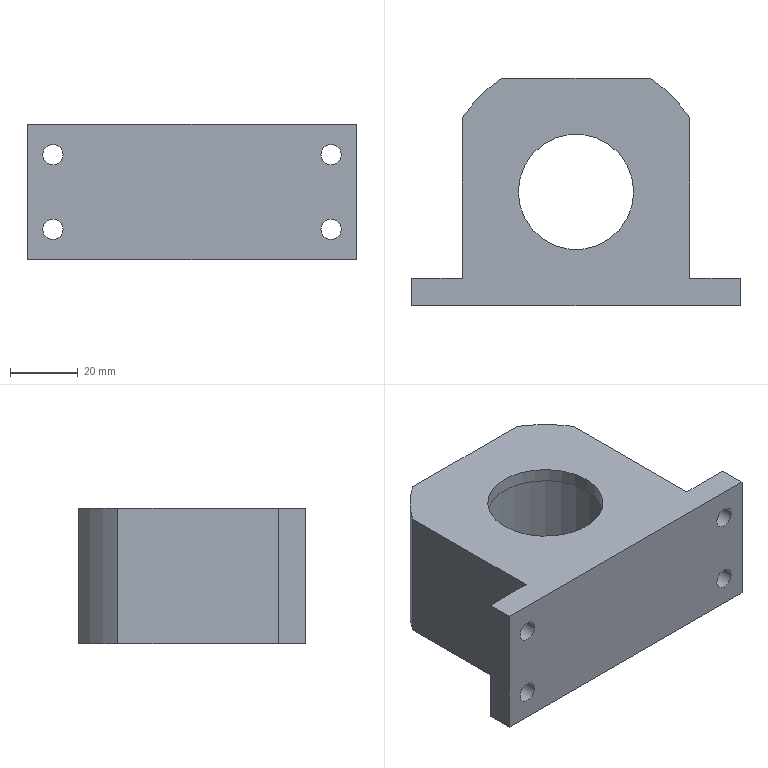Part | STEP file | Cut-off module bearing seat | 1 solid | 41 faces | box 97 x 67 x 40 mm | volume 117140 mm3 | cylinder 22 | plane 11 | cone 8 | commonest cylinder face diameters 3.3 x8 6 x8 34 x2 47 x2 80 x2
STEP:
#1=CARTESIAN_POINT('',(22.863,21.213,10.1));
#2=VERTEX_POINT('',#1);
#3=CARTESIAN_POINT('',(19.563,21.213,10.1));
#4=VERTEX_POINT('',#3);
#5=CARTESIAN_POINT('',(21.213,21.213,10.1));
#6=DIRECTION('',(0.,0.,-1.));
#7=DIRECTION('',(-1.,0.,0.));
#8=AXIS2_PLACEMENT_3D('',#5,#6,#7);
#9=CIRCLE('',#8,1.65);
#10=EDGE_CURVE('',#2,#4,#9,.T.);
#11=ORIENTED_EDGE('',*,*,#10,.F.);
#12=CARTESIAN_POINT('',(22.863,21.213,0.));
#13=VERTEX_POINT('',#12);
#14=CARTESIAN_POINT('',(22.863,21.213,0.));
#15=DIRECTION('',(0.,0.,-1.));
#16=VECTOR('',#15,1000.);
#17=LINE('',#14,#16);
#18=EDGE_CURVE('',#2,#13,#17,.T.);
#19=ORIENTED_EDGE('',*,*,#18,.T.);
#20=CARTESIAN_POINT('',(19.563,21.213,0.));
#21=VERTEX_POINT('',#20);
#22=CARTESIAN_POINT('',(21.213,21.213,0.));
#23=DIRECTION('',(0.,0.,-1.));
#24=DIRECTION('',(-1.,0.,0.));
#25=AXIS2_PLACEMENT_3D('',#22,#23,#24);
#26=CIRCLE('',#25,1.65);
#27=EDGE_CURVE('',#13,#21,#26,.T.);
#28=ORIENTED_EDGE('',*,*,#27,.T.);
#29=CARTESIAN_POINT('',(19.563,21.213,0.));
#30=DIRECTION('',(0.,0.,-1.));
#31=VECTOR('',#30,1000.);
#32=LINE('',#29,#31);
#33=EDGE_CURVE('',#4,#21,#32,.T.);
#34=ORIENTED_EDGE('',*,*,#33,.F.);
#35=EDGE_LOOP('',(#11,#19,#28,#34));
#36=FACE_OUTER_BOUND('',#35,.T.);
#37=CARTESIAN_POINT('',(21.213,21.213,0.));
#38=DIRECTION('',(0.,0.,-1.));
#39=DIRECTION('',(-1.,0.,0.));
#40=AXIS2_PLACEMENT_3D('',#37,#38,#39);
#41=CYLINDRICAL_SURFACE('',#40,1.65);
#42=ADVANCED_FACE('',(#36),#41,.F.);
#43=CARTESIAN_POINT('',(21.213,21.213,11.091));
#44=VERTEX_POINT('',#43);
#45=CARTESIAN_POINT('',(19.563,21.213,10.1));
#46=DIRECTION('',(-0.8572,0.,-0.515));
#47=VECTOR('',#46,1000.);
#48=LINE('',#45,#47);
#49=EDGE_CURVE('',#44,#4,#48,.T.);
#50=ORIENTED_EDGE('',*,*,#49,.F.);
#51=CARTESIAN_POINT('',(22.863,21.213,10.1));
#52=DIRECTION('',(0.8572,0.,-0.515));
#53=VECTOR('',#52,1000.);
#54=LINE('',#51,#53);
#55=EDGE_CURVE('',#44,#2,#54,.T.);
#56=ORIENTED_EDGE('',*,*,#55,.T.);
#57=ORIENTED_EDGE('',*,*,#10,.T.);
#58=EDGE_LOOP('',(#50,#56,#57));
#59=FACE_OUTER_BOUND('',#58,.T.);
#60=CARTESIAN_POINT('',(21.213,21.213,10.1));
#61=DIRECTION('',(0.,0.,-1.));
#62=DIRECTION('',(-1.,0.,0.));
#63=AXIS2_PLACEMENT_3D('',#60,#61,#62);
#64=CONICAL_SURFACE('',#63,1.65,1.03);
#65=ADVANCED_FACE('',(#59),#64,.F.);
#66=CARTESIAN_POINT('',(-19.563,21.213,10.1));
#67=VERTEX_POINT('',#66);
#68=CARTESIAN_POINT('',(-22.863,21.213,10.1));
#69=VERTEX_POINT('',#68);
#70=CARTESIAN_POINT('',(-21.213,21.213,10.1));
#71=DIRECTION('',(0.,0.,-1.));
#72=DIRECTION('',(-1.,0.,0.));
#73=AXIS2_PLACEMENT_3D('',#70,#71,#72);
#74=CIRCLE('',#73,1.65);
#75=EDGE_CURVE('',#67,#69,#74,.T.);
#76=ORIENTED_EDGE('',*,*,#75,.F.);
#77=CARTESIAN_POINT('',(-19.563,21.213,0.));
#78=VERTEX_POINT('',#77);
#79=CARTESIAN_POINT('',(-19.563,21.213,0.));
#80=DIRECTION('',(0.,0.,-1.));
#81=VECTOR('',#80,1000.);
#82=LINE('',#79,#81);
#83=EDGE_CURVE('',#67,#78,#82,.T.);
#84=ORIENTED_EDGE('',*,*,#83,.T.);
#85=CARTESIAN_POINT('',(-22.863,21.213,0.));
#86=VERTEX_POINT('',#85);
#87=CARTESIAN_POINT('',(-21.213,21.213,0.));
#88=DIRECTION('',(0.,0.,-1.));
#89=DIRECTION('',(-1.,0.,0.));
#90=AXIS2_PLACEMENT_3D('',#87,#88,#89);
#91=CIRCLE('',#90,1.65);
#92=EDGE_CURVE('',#78,#86,#91,.T.);
#93=ORIENTED_EDGE('',*,*,#92,.T.);
#94=CARTESIAN_POINT('',(-22.863,21.213,0.));
#95=DIRECTION('',(0.,0.,-1.));
#96=VECTOR('',#95,1000.);
#97=LINE('',#94,#96);
#98=EDGE_CURVE('',#69,#86,#97,.T.);
#99=ORIENTED_EDGE('',*,*,#98,.F.);
#100=EDGE_LOOP('',(#76,#84,#93,#99));
#101=FACE_OUTER_BOUND('',#100,.T.);
#102=CARTESIAN_POINT('',(-21.213,21.213,0.));
#103=DIRECTION('',(0.,0.,-1.));
#104=DIRECTION('',(-1.,0.,0.));
#105=AXIS2_PLACEMENT_3D('',#102,#103,#104);
#106=CYLINDRICAL_SURFACE('',#105,1.65);
#107=ADVANCED_FACE('',(#101),#106,.F.);
#108=CARTESIAN_POINT('',(-21.213,21.213,11.091));
#109=VERTEX_POINT('',#108);
#110=CARTESIAN_POINT('',(-22.863,21.213,10.1));
#111=DIRECTION('',(-0.8572,0.,-0.515));
#112=VECTOR('',#111,1000.);
#113=LINE('',#110,#112);
#114=EDGE_CURVE('',#109,#69,#113,.T.);
#115=ORIENTED_EDGE('',*,*,#114,.F.);
#116=CARTESIAN_POINT('',(-19.563,21.213,10.1));
#117=DIRECTION('',(0.8572,0.,-0.515));
#118=VECTOR('',#117,1000.);
#119=LINE('',#116,#118);
#120=EDGE_CURVE('',#109,#67,#119,.T.);
#121=ORIENTED_EDGE('',*,*,#120,.T.);
#122=ORIENTED_EDGE('',*,*,#75,.T.);
#123=EDGE_LOOP('',(#115,#121,#122));
#124=FACE_OUTER_BOUND('',#123,.T.);
#125=CARTESIAN_POINT('',(-21.213,21.213,10.1));
#126=DIRECTION('',(0.,0.,-1.));
#127=DIRECTION('',(-1.,0.,0.));
#128=AXIS2_PLACEMENT_3D('',#125,#126,#127);
#129=CONICAL_SURFACE('',#128,1.65,1.03);
#130=ADVANCED_FACE('',(#124),#129,.F.);
#131=CARTESIAN_POINT('',(-19.563,-21.213,10.1));
#132=VERTEX_POINT('',#131);
#133=CARTESIAN_POINT('',(-22.863,-21.213,10.1));
#134=VERTEX_POINT('',#133);
#135=CARTESIAN_POINT('',(-21.213,-21.213,10.1));
#136=DIRECTION('',(0.,0.,-1.));
#137=DIRECTION('',(-1.,0.,0.));
#138=AXIS2_PLACEMENT_3D('',#135,#136,#137);
#139=CIRCLE('',#138,1.65);
#140=EDGE_CURVE('',#132,#134,#139,.T.);
#141=ORIENTED_EDGE('',*,*,#140,.F.);
#142=CARTESIAN_POINT('',(-19.563,-21.213,0.));
#143=VERTEX_POINT('',#142);
#144=CARTESIAN_POINT('',(-19.563,-21.213,0.));
#145=DIRECTION('',(0.,0.,-1.));
#146=VECTOR('',#145,1000.);
#147=LINE('',#144,#146);
#148=EDGE_CURVE('',#132,#143,#147,.T.);
#149=ORIENTED_EDGE('',*,*,#148,.T.);
#150=CARTESIAN_POINT('',(-22.863,-21.213,0.));
#151=VERTEX_POINT('',#150);
#152=CARTESIAN_POINT('',(-21.213,-21.213,0.));
#153=DIRECTION('',(0.,0.,-1.));
#154=DIRECTION('',(-1.,0.,0.));
#155=AXIS2_PLACEMENT_3D('',#152,#153,#154);
#156=CIRCLE('',#155,1.65);
#157=EDGE_CURVE('',#143,#151,#156,.T.);
#158=ORIENTED_EDGE('',*,*,#157,.T.);
#159=CARTESIAN_POINT('',(-22.863,-21.213,0.));
#160=DIRECTION('',(0.,0.,-1.));
#161=VECTOR('',#160,1000.);
#162=LINE('',#159,#161);
#163=EDGE_CURVE('',#134,#151,#162,.T.);
#164=ORIENTED_EDGE('',*,*,#163,.F.);
#165=EDGE_LOOP('',(#141,#149,#158,#164));
#166=FACE_OUTER_BOUND('',#165,.T.);
#167=CARTESIAN_POINT('',(-21.213,-21.213,0.));
#168=DIRECTION('',(0.,0.,-1.));
#169=DIRECTION('',(-1.,0.,0.));
#170=AXIS2_PLACEMENT_3D('',#167,#168,#169);
#171=CYLINDRICAL_SURFACE('',#170,1.65);
#172=ADVANCED_FACE('',(#166),#171,.F.);
#173=CARTESIAN_POINT('',(-21.213,-21.213,11.091));
#174=VERTEX_POINT('',#173);
#175=CARTESIAN_POINT('',(-22.863,-21.213,10.1));
#176=DIRECTION('',(-0.8572,0.,-0.515));
#177=VECTOR('',#176,1000.);
#178=LINE('',#175,#177);
#179=EDGE_CURVE('',#174,#134,#178,.T.);
#180=ORIENTED_EDGE('',*,*,#179,.F.);
#181=CARTESIAN_POINT('',(-19.563,-21.213,10.1));
#182=DIRECTION('',(0.8572,0.,-0.515));
#183=VECTOR('',#182,1000.);
#184=LINE('',#181,#183);
#185=EDGE_CURVE('',#174,#132,#184,.T.);
#186=ORIENTED_EDGE('',*,*,#185,.T.);
#187=ORIENTED_EDGE('',*,*,#140,.T.);
#188=EDGE_LOOP('',(#180,#186,#187));
#189=FACE_OUTER_BOUND('',#188,.T.);
#190=CARTESIAN_POINT('',(-21.213,-21.213,10.1));
#191=DIRECTION('',(0.,0.,-1.));
#192=DIRECTION('',(-1.,0.,0.));
#193=AXIS2_PLACEMENT_3D('',#190,#191,#192);
#194=CONICAL_SURFACE('',#193,1.65,1.03);
#195=ADVANCED_FACE('',(#189),#194,.F.);
#196=CARTESIAN_POINT('',(22.863,-21.213,10.1));
#197=VERTEX_POINT('',#196);
#198=CARTESIAN_POINT('',(19.563,-21.213,10.1));
#199=VERTEX_POINT('',#198);
#200=CARTESIAN_POINT('',(21.213,-21.213,10.1));
#201=DIRECTION('',(0.,0.,-1.));
#202=DIRECTION('',(-1.,0.,0.));
#203=AXIS2_PLACEMENT_3D('',#200,#201,#202);
#204=CIRCLE('',#203,1.65);
#205=EDGE_CURVE('',#197,#199,#204,.T.);
#206=ORIENTED_EDGE('',*,*,#205,.F.);
#207=CARTESIAN_POINT('',(22.863,-21.213,0.));
#208=VERTEX_POINT('',#207);
#209=CARTESIAN_POINT('',(22.863,-21.213,0.));
#210=DIRECTION('',(0.,0.,-1.));
#211=VECTOR('',#210,1000.);
#212=LINE('',#209,#211);
#213=EDGE_CURVE('',#197,#208,#212,.T.);
#214=ORIENTED_EDGE('',*,*,#213,.T.);
#215=CARTESIAN_POINT('',(19.563,-21.213,0.));
#216=VERTEX_POINT('',#215);
#217=CARTESIAN_POINT('',(21.213,-21.213,0.));
#218=DIRECTION('',(0.,0.,-1.));
#219=DIRECTION('',(-1.,0.,0.));
#220=AXIS2_PLACEMENT_3D('',#217,#218,#219);
#221=CIRCLE('',#220,1.65);
#222=EDGE_CURVE('',#208,#216,#221,.T.);
#223=ORIENTED_EDGE('',*,*,#222,.T.);
#224=CARTESIAN_POINT('',(19.563,-21.213,0.));
#225=DIRECTION('',(0.,0.,-1.));
#226=VECTOR('',#225,1000.);
#227=LINE('',#224,#226);
#228=EDGE_CURVE('',#199,#216,#227,.T.);
#229=ORIENTED_EDGE('',*,*,#228,.F.);
#230=EDGE_LOOP('',(#206,#214,#223,#229));
#231=FACE_OUTER_BOUND('',#230,.T.);
#232=CARTESIAN_POINT('',(21.213,-21.213,0.));
#233=DIRECTION('',(0.,0.,-1.));
#234=DIRECTION('',(-1.,0.,0.));
#235=AXIS2_PLACEMENT_3D('',#232,#233,#234);
#236=CYLINDRICAL_SURFACE('',#235,1.65);
#237=ADVANCED_FACE('',(#231),#236,.F.);
#238=CARTESIAN_POINT('',(21.213,-21.213,11.091));
#239=VERTEX_POINT('',#238);
#240=CARTESIAN_POINT('',(19.563,-21.213,10.1));
#241=DIRECTION('',(-0.8572,0.,-0.515));
#242=VECTOR('',#241,1000.);
#243=LINE('',#240,#242);
#244=EDGE_CURVE('',#239,#199,#243,.T.);
#245=ORIENTED_EDGE('',*,*,#244,.F.);
#246=CARTESIAN_POINT('',(22.863,-21.213,10.1));
#247=DIRECTION('',(0.8572,0.,-0.515));
#248=VECTOR('',#247,1000.);
#249=LINE('',#246,#248);
#250=EDGE_CURVE('',#239,#197,#249,.T.);
#251=ORIENTED_EDGE('',*,*,#250,.T.);
#252=ORIENTED_EDGE('',*,*,#205,.T.);
#253=EDGE_LOOP('',(#245,#251,#252));
#254=FACE_OUTER_BOUND('',#253,.T.);
#255=CARTESIAN_POINT('',(21.213,-21.213,10.1));
#256=DIRECTION('',(0.,0.,-1.));
#257=DIRECTION('',(-1.,0.,0.));
#258=AXIS2_PLACEMENT_3D('',#255,#256,#257);
#259=CONICAL_SURFACE('',#258,1.65,1.03);
#260=ADVANCED_FACE('',(#254),#259,.F.);
#261=CARTESIAN_POINT('',(-44.,-33.5,9.));
#262=VERTEX_POINT('',#261);
#263=CARTESIAN_POINT('',(-38.,-33.5,9.));
#264=VERTEX_POINT('',#263);
#265=CARTESIAN_POINT('',(-41.,-33.5,9.));
#266=DIRECTION('',(0.,-1.,0.));
#267=DIRECTION('',(0.,0.,1.));
#268=AXIS2_PLACEMENT_3D('',#265,#266,#267);
#269=CIRCLE('',#268,3.);
#270=EDGE_CURVE('',#262,#264,#269,.T.);
#271=ORIENTED_EDGE('',*,*,#270,.T.);
#272=CARTESIAN_POINT('',(-38.,-25.5,9.));
#273=VERTEX_POINT('',#272);
#274=CARTESIAN_POINT('',(-38.,-45.5,9.));
#275=DIRECTION('',(0.,1.,0.));
#276=VECTOR('',#275,1000.);
#277=LINE('',#274,#276);
#278=EDGE_CURVE('',#264,#273,#277,.T.);
#279=ORIENTED_EDGE('',*,*,#278,.T.);
#280=CARTESIAN_POINT('',(-44.,-25.5,9.));
#281=VERTEX_POINT('',#280);
#282=CARTESIAN_POINT('',(-41.,-25.5,9.));
#283=DIRECTION('',(0.,-1.,0.));
#284=DIRECTION('',(1.,0.,0.));
#285=AXIS2_PLACEMENT_3D('',#282,#283,#284);
#286=CIRCLE('',#285,3.);
#287=EDGE_CURVE('',#281,#273,#286,.T.);
#288=ORIENTED_EDGE('',*,*,#287,.F.);
#289=CARTESIAN_POINT('',(-44.,-45.5,9.));
#290=DIRECTION('',(0.,1.,0.));
#291=VECTOR('',#290,1000.);
#292=LINE('',#289,#291);
#293=EDGE_CURVE('',#262,#281,#292,.T.);
#294=ORIENTED_EDGE('',*,*,#293,.F.);
#295=EDGE_LOOP('',(#271,#279,#288,#294));
#296=FACE_OUTER_BOUND('',#295,.T.);
#297=CARTESIAN_POINT('',(-41.,-45.5,9.));
#298=DIRECTION('',(0.,1.,0.));
#299=DIRECTION('',(-1.,0.,0.));
#300=AXIS2_PLACEMENT_3D('',#297,#298,#299);
#301=CYLINDRICAL_SURFACE('',#300,3.);
#302=ADVANCED_FACE('',(#296),#301,.F.);
#303=CARTESIAN_POINT('',(-44.,-33.5,31.));
#304=VERTEX_POINT('',#303);
#305=CARTESIAN_POINT('',(-38.,-33.5,31.));
#306=VERTEX_POINT('',#305);
#307=CARTESIAN_POINT('',(-41.,-33.5,31.));
#308=DIRECTION('',(0.,-1.,0.));
#309=DIRECTION('',(0.,0.,1.));
#310=AXIS2_PLACEMENT_3D('',#307,#308,#309);
#311=CIRCLE('',#310,3.);
#312=EDGE_CURVE('',#304,#306,#311,.T.);
#313=ORIENTED_EDGE('',*,*,#312,.T.);
#314=CARTESIAN_POINT('',(-38.,-25.5,31.));
#315=VERTEX_POINT('',#314);
#316=CARTESIAN_POINT('',(-38.,-45.5,31.));
#317=DIRECTION('',(0.,1.,0.));
#318=VECTOR('',#317,1000.);
#319=LINE('',#316,#318);
#320=EDGE_CURVE('',#306,#315,#319,.T.);
#321=ORIENTED_EDGE('',*,*,#320,.T.);
#322=CARTESIAN_POINT('',(-44.,-25.5,31.));
#323=VERTEX_POINT('',#322);
#324=CARTESIAN_POINT('',(-41.,-25.5,31.));
#325=DIRECTION('',(0.,-1.,0.));
#326=DIRECTION('',(1.,0.,0.));
#327=AXIS2_PLACEMENT_3D('',#324,#325,#326);
#328=CIRCLE('',#327,3.);
#329=EDGE_CURVE('',#323,#315,#328,.T.);
#330=ORIENTED_EDGE('',*,*,#329,.F.);
#331=CARTESIAN_POINT('',(-44.,-45.5,31.));
#332=DIRECTION('',(0.,1.,0.));
#333=VECTOR('',#332,1000.);
#334=LINE('',#331,#333);
#335=EDGE_CURVE('',#304,#323,#334,.T.);
#336=ORIENTED_EDGE('',*,*,#335,.F.);
#337=EDGE_LOOP('',(#313,#321,#330,#336));
#338=FACE_OUTER_BOUND('',#337,.T.);
#339=CARTESIAN_POINT('',(-41.,-45.5,31.));
#340=DIRECTION('',(0.,1.,0.));
#341=DIRECTION('',(-1.,0.,0.));
#342=AXIS2_PLACEMENT_3D('',#339,#340,#341);
#343=CYLINDRICAL_SURFACE('',#342,3.);
#344=ADVANCED_FACE('',(#338),#343,.F.);
#345=CARTESIAN_POINT('',(44.,-33.5,9.));
#346=VERTEX_POINT('',#345);
#347=CARTESIAN_POINT('',(38.,-33.5,9.));
#348=VERTEX_POINT('',#347);
#349=CARTESIAN_POINT('',(41.,-33.5,9.));
#350=DIRECTION('',(0.,1.,0.));
#351=DIRECTION('',(0.,0.,1.));
#352=AXIS2_PLACEMENT_3D('',#349,#350,#351);
#353=CIRCLE('',#352,3.);
#354=EDGE_CURVE('',#346,#348,#353,.T.);
#355=ORIENTED_EDGE('',*,*,#354,.F.);
#356=CARTESIAN_POINT('',(44.,-25.5,9.));
#357=VERTEX_POINT('',#356);
#358=CARTESIAN_POINT('',(44.,-45.5,9.));
#359=DIRECTION('',(0.,1.,0.));
#360=VECTOR('',#359,1000.);
#361=LINE('',#358,#360);
#362=EDGE_CURVE('',#346,#357,#361,.T.);
#363=ORIENTED_EDGE('',*,*,#362,.T.);
#364=CARTESIAN_POINT('',(38.,-25.5,9.));
#365=VERTEX_POINT('',#364);
#366=CARTESIAN_POINT('',(41.,-25.5,9.));
#367=DIRECTION('',(0.,1.,0.));
#368=DIRECTION('',(-1.,0.,0.));
#369=AXIS2_PLACEMENT_3D('',#366,#367,#368);
#370=CIRCLE('',#369,3.);
#371=EDGE_CURVE('',#357,#365,#370,.T.);
#372=ORIENTED_EDGE('',*,*,#371,.T.);
#373=CARTESIAN_POINT('',(38.,-45.5,9.));
#374=DIRECTION('',(0.,1.,0.));
#375=VECTOR('',#374,1000.);
#376=LINE('',#373,#375);
#377=EDGE_CURVE('',#348,#365,#376,.T.);
#378=ORIENTED_EDGE('',*,*,#377,.F.);
#379=EDGE_LOOP('',(#355,#363,#372,#378));
#380=FACE_OUTER_BOUND('',#379,.T.);
#381=CARTESIAN_POINT('',(41.,-45.5,9.));
#382=DIRECTION('',(0.,1.,0.));
#383=DIRECTION('',(-1.,0.,0.));
#384=AXIS2_PLACEMENT_3D('',#381,#382,#383);
#385=CYLINDRICAL_SURFACE('',#384,3.);
#386=ADVANCED_FACE('',(#380),#385,.F.);
#387=CARTESIAN_POINT('',(44.,-33.5,31.));
#388=VERTEX_POINT('',#387);
#389=CARTESIAN_POINT('',(38.,-33.5,31.));
#390=VERTEX_POINT('',#389);
#391=CARTESIAN_POINT('',(41.,-33.5,31.));
#392=DIRECTION('',(0.,1.,0.));
#393=DIRECTION('',(0.,0.,1.));
#394=AXIS2_PLACEMENT_3D('',#391,#392,#393);
#395=CIRCLE('',#394,3.);
#396=EDGE_CURVE('',#388,#390,#395,.T.);
#397=ORIENTED_EDGE('',*,*,#396,.F.);
#398=CARTESIAN_POINT('',(44.,-25.5,31.));
#399=VERTEX_POINT('',#398);
#400=CARTESIAN_POINT('',(44.,-45.5,31.));
#401=DIRECTION('',(0.,1.,0.));
#402=VECTOR('',#401,1000.);
#403=LINE('',#400,#402);
#404=EDGE_CURVE('',#388,#399,#403,.T.);
#405=ORIENTED_EDGE('',*,*,#404,.T.);
#406=CARTESIAN_POINT('',(38.,-25.5,31.));
#407=VERTEX_POINT('',#406);
#408=CARTESIAN_POINT('',(41.,-25.5,31.));
#409=DIRECTION('',(0.,1.,0.));
#410=DIRECTION('',(-1.,0.,0.));
#411=AXIS2_PLACEMENT_3D('',#408,#409,#410);
#412=CIRCLE('',#411,3.);
#413=EDGE_CURVE('',#399,#407,#412,.T.);
#414=ORIENTED_EDGE('',*,*,#413,.T.);
#415=CARTESIAN_POINT('',(38.,-45.5,31.));
#416=DIRECTION('',(0.,1.,0.));
#417=VECTOR('',#416,1000.);
#418=LINE('',#415,#417);
#419=EDGE_CURVE('',#390,#407,#418,.T.);
#420=ORIENTED_EDGE('',*,*,#419,.F.);
#421=EDGE_LOOP('',(#397,#405,#414,#420));
#422=FACE_OUTER_BOUND('',#421,.T.);
#423=CARTESIAN_POINT('',(41.,-45.5,31.));
#424=DIRECTION('',(0.,1.,0.));
#425=DIRECTION('',(-1.,0.,0.));
#426=AXIS2_PLACEMENT_3D('',#423,#424,#425);
#427=CYLINDRICAL_SURFACE('',#426,3.);
#428=ADVANCED_FACE('',(#422),#427,.F.);
#429=CARTESIAN_POINT('',(-17.,0.,36.));
#430=VERTEX_POINT('',#429);
#431=CARTESIAN_POINT('',(17.,0.,36.));
#432=VERTEX_POINT('',#431);
#433=CARTESIAN_POINT('',(0.,0.,36.));
#434=DIRECTION('',(0.,0.,1.));
#435=DIRECTION('',(1.,0.,0.));
#436=AXIS2_PLACEMENT_3D('',#433,#434,#435);
#437=CIRCLE('',#436,17.);
#438=EDGE_CURVE('',#430,#432,#437,.T.);
#439=ORIENTED_EDGE('',*,*,#438,.F.);
#440=CARTESIAN_POINT('',(-17.,0.,40.));
#441=VERTEX_POINT('',#440);
#442=CARTESIAN_POINT('',(-17.,0.,36.));
#443=DIRECTION('',(0.,0.,1.));
#444=VECTOR('',#443,1000.);
#445=LINE('',#442,#444);
#446=EDGE_CURVE('',#430,#441,#445,.T.);
#447=ORIENTED_EDGE('',*,*,#446,.T.);
#448=CARTESIAN_POINT('',(17.,0.,40.));
#449=VERTEX_POINT('',#448);
#450=CARTESIAN_POINT('',(0.,0.,40.));
#451=DIRECTION('',(0.,0.,1.));
#452=DIRECTION('',(1.,0.,0.));
#453=AXIS2_PLACEMENT_3D('',#450,#451,#452);
#454=CIRCLE('',#453,17.);
#455=EDGE_CURVE('',#441,#449,#454,.T.);
#456=ORIENTED_EDGE('',*,*,#455,.T.);
#457=CARTESIAN_POINT('',(17.,0.,36.));
#458=DIRECTION('',(0.,0.,1.));
#459=VECTOR('',#458,1000.);
#460=LINE('',#457,#459);
#461=EDGE_CURVE('',#432,#449,#460,.T.);
#462=ORIENTED_EDGE('',*,*,#461,.F.);
#463=EDGE_LOOP('',(#439,#447,#456,#462));
#464=FACE_OUTER_BOUND('',#463,.T.);
#465=CARTESIAN_POINT('',(0.,0.,36.));
#466=DIRECTION('',(0.,0.,1.));
#467=DIRECTION('',(1.,0.,0.));
#468=AXIS2_PLACEMENT_3D('',#465,#466,#467);
#469=CYLINDRICAL_SURFACE('',#468,17.);
#470=ADVANCED_FACE('',(#464),#469,.F.);
#471=CARTESIAN_POINT('',(-23.5,0.,36.));
#472=VERTEX_POINT('',#471);
#473=CARTESIAN_POINT('',(23.5,0.,36.));
#474=VERTEX_POINT('',#473);
#475=CARTESIAN_POINT('',(0.,0.,36.));
#476=DIRECTION('',(0.,0.,1.));
#477=DIRECTION('',(1.,0.,0.));
#478=AXIS2_PLACEMENT_3D('',#475,#476,#477);
#479=CIRCLE('',#478,23.5);
#480=EDGE_CURVE('',#472,#474,#479,.T.);
#481=ORIENTED_EDGE('',*,*,#480,.T.);
#482=CARTESIAN_POINT('',(23.5,0.,0.));
#483=VERTEX_POINT('',#482);
#484=CARTESIAN_POINT('',(23.5,0.,40.));
#485=DIRECTION('',(0.,0.,-1.));
#486=VECTOR('',#485,1000.);
#487=LINE('',#484,#486);
#488=EDGE_CURVE('',#474,#483,#487,.T.);
#489=ORIENTED_EDGE('',*,*,#488,.T.);
#490=CARTESIAN_POINT('',(-23.5,0.,0.));
#491=VERTEX_POINT('',#490);
#492=CARTESIAN_POINT('',(0.,0.,0.));
#493=DIRECTION('',(0.,0.,1.));
#494=DIRECTION('',(1.,0.,0.));
#495=AXIS2_PLACEMENT_3D('',#492,#493,#494);
#496=CIRCLE('',#495,23.5);
#497=EDGE_CURVE('',#491,#483,#496,.T.);
#498=ORIENTED_EDGE('',*,*,#497,.F.);
#499=CARTESIAN_POINT('',(-23.5,0.,40.));
#500=DIRECTION('',(0.,0.,-1.));
#501=VECTOR('',#500,1000.);
#502=LINE('',#499,#501);
#503=EDGE_CURVE('',#472,#491,#502,.T.);
#504=ORIENTED_EDGE('',*,*,#503,.F.);
#505=EDGE_LOOP('',(#481,#489,#498,#504));
#506=FACE_OUTER_BOUND('',#505,.T.);
#507=CARTESIAN_POINT('',(0.,0.,40.));
#508=DIRECTION('',(0.,0.,-1.));
#509=DIRECTION('',(-1.,0.,0.));
#510=AXIS2_PLACEMENT_3D('',#507,#508,#509);
#511=CYLINDRICAL_SURFACE('',#510,23.5);
#512=ADVANCED_FACE('',(#506),#511,.F.);
#513=CARTESIAN_POINT('',(0.,0.,40.));
#514=DIRECTION('',(0.,0.,1.));
#515=DIRECTION('',(1.,0.,0.));
#516=AXIS2_PLACEMENT_3D('',#513,#514,#515);
#517=CIRCLE('',#516,17.);
#518=EDGE_CURVE('',#449,#441,#517,.T.);
#519=ORIENTED_EDGE('',*,*,#518,.F.);
#520=ORIENTED_EDGE('',*,*,#455,.F.);
#521=EDGE_LOOP('',(#519,#520));
#522=FACE_BOUND('',#521,.T.);
#523=CARTESIAN_POINT('',(21.857,33.5,40.));
#524=VERTEX_POINT('',#523);
#525=CARTESIAN_POINT('',(33.5,21.857,40.));
#526=VERTEX_POINT('',#525);
#527=CARTESIAN_POINT('',(0.,0.,40.));
#528=DIRECTION('',(0.,0.,-1.));
#529=DIRECTION('',(1.,0.,0.));
#530=AXIS2_PLACEMENT_3D('',#527,#528,#529);
#531=CIRCLE('',#530,40.);
#532=EDGE_CURVE('',#524,#526,#531,.T.);
#533=ORIENTED_EDGE('',*,*,#532,.F.);
#534=CARTESIAN_POINT('',(-21.857,33.5,40.));
#535=VERTEX_POINT('',#534);
#536=CARTESIAN_POINT('',(-33.5,33.5,40.));
#537=DIRECTION('',(-1.,0.,0.));
#538=VECTOR('',#537,1000.);
#539=LINE('',#536,#538);
#540=EDGE_CURVE('',#524,#535,#539,.T.);
#541=ORIENTED_EDGE('',*,*,#540,.T.);
#542=CARTESIAN_POINT('',(-33.5,21.857,40.));
#543=VERTEX_POINT('',#542);
#544=CARTESIAN_POINT('',(0.,0.,40.));
#545=DIRECTION('',(0.,0.,-1.));
#546=DIRECTION('',(1.,0.,0.));
#547=AXIS2_PLACEMENT_3D('',#544,#545,#546);
#548=CIRCLE('',#547,40.);
#549=EDGE_CURVE('',#543,#535,#548,.T.);
#550=ORIENTED_EDGE('',*,*,#549,.F.);
#551=CARTESIAN_POINT('',(-33.5,-25.5,40.));
#552=VERTEX_POINT('',#551);
#553=CARTESIAN_POINT('',(-33.5,33.5,40.));
#554=DIRECTION('',(0.,-1.,0.));
#555=VECTOR('',#554,1000.);
#556=LINE('',#553,#555);
#557=EDGE_CURVE('',#543,#552,#556,.T.);
#558=ORIENTED_EDGE('',*,*,#557,.T.);
#559=CARTESIAN_POINT('',(-48.5,-25.5,40.));
#560=VERTEX_POINT('',#559);
#561=CARTESIAN_POINT('',(-48.5,-25.5,40.));
#562=DIRECTION('',(1.,0.,0.));
#563=VECTOR('',#562,1000.);
#564=LINE('',#561,#563);
#565=EDGE_CURVE('',#560,#552,#564,.T.);
#566=ORIENTED_EDGE('',*,*,#565,.F.);
#567=CARTESIAN_POINT('',(-48.5,-33.5,40.));
#568=VERTEX_POINT('',#567);
#569=CARTESIAN_POINT('',(-48.5,-33.5,40.));
#570=DIRECTION('',(0.,-1.,0.));
#571=VECTOR('',#570,1000.);
#572=LINE('',#569,#571);
#573=EDGE_CURVE('',#560,#568,#572,.T.);
#574=ORIENTED_EDGE('',*,*,#573,.T.);
#575=CARTESIAN_POINT('',(48.5,-33.5,40.));
#576=VERTEX_POINT('',#575);
#577=CARTESIAN_POINT('',(-33.5,-33.5,40.));
#578=DIRECTION('',(1.,0.,0.));
#579=VECTOR('',#578,1000.);
#580=LINE('',#577,#579);
#581=EDGE_CURVE('',#568,#576,#580,.T.);
#582=ORIENTED_EDGE('',*,*,#581,.T.);
#583=CARTESIAN_POINT('',(48.5,-25.5,40.));
#584=VERTEX_POINT('',#583);
#585=CARTESIAN_POINT('',(48.5,-33.5,40.));
#586=DIRECTION('',(0.,-1.,0.));
#587=VECTOR('',#586,1000.);
#588=LINE('',#585,#587);
#589=EDGE_CURVE('',#584,#576,#588,.T.);
#590=ORIENTED_EDGE('',*,*,#589,.F.);
#591=CARTESIAN_POINT('',(33.5,-25.5,40.));
#592=VERTEX_POINT('',#591);
#593=CARTESIAN_POINT('',(48.5,-25.5,40.));
#594=DIRECTION('',(-1.,0.,0.));
#595=VECTOR('',#594,1000.);
#596=LINE('',#593,#595);
#597=EDGE_CURVE('',#584,#592,#596,.T.);
#598=ORIENTED_EDGE('',*,*,#597,.T.);
#599=CARTESIAN_POINT('',(33.5,33.5,40.));
#600=DIRECTION('',(0.,1.,0.));
#601=VECTOR('',#600,1000.);
#602=LINE('',#599,#601);
#603=EDGE_CURVE('',#592,#526,#602,.T.);
#604=ORIENTED_EDGE('',*,*,#603,.T.);
#605=EDGE_LOOP('',(#533,#541,#550,#558,#566,#574,#582,#590,#598,#604));
#606=FACE_OUTER_BOUND('',#605,.T.);
#607=CARTESIAN_POINT('',(0.,0.,40.));
#608=DIRECTION('',(0.,0.,1.));
#609=DIRECTION('',(1.,0.,0.));
#610=AXIS2_PLACEMENT_3D('',#607,#608,#609);
#611=PLANE('',#610);
#612=ADVANCED_FACE('',(#522,#606),#611,.T.);
#613=CARTESIAN_POINT('',(21.213,21.213,0.));
#614=DIRECTION('',(0.,0.,-1.));
#615=DIRECTION('',(-1.,0.,0.));
#616=AXIS2_PLACEMENT_3D('',#613,#614,#615);
#617=CIRCLE('',#616,1.65);
#618=EDGE_CURVE('',#21,#13,#617,.T.);
#619=ORIENTED_EDGE('',*,*,#618,.F.);
#620=ORIENTED_EDGE('',*,*,#27,.F.);
#621=EDGE_LOOP('',(#619,#620));
#622=FACE_BOUND('',#621,.T.);
#623=CARTESIAN_POINT('',(-21.213,21.213,0.));
#624=DIRECTION('',(0.,0.,-1.));
#625=DIRECTION('',(-1.,0.,0.));
#626=AXIS2_PLACEMENT_3D('',#623,#624,#625);
#627=CIRCLE('',#626,1.65);
#628=EDGE_CURVE('',#86,#78,#627,.T.);
#629=ORIENTED_EDGE('',*,*,#628,.F.);
#630=ORIENTED_EDGE('',*,*,#92,.F.);
#631=EDGE_LOOP('',(#629,#630));
#632=FACE_BOUND('',#631,.T.);
#633=CARTESIAN_POINT('',(-21.213,-21.213,0.));
#634=DIRECTION('',(0.,0.,-1.));
#635=DIRECTION('',(-1.,0.,0.));
#636=AXIS2_PLACEMENT_3D('',#633,#634,#635);
#637=CIRCLE('',#636,1.65);
#638=EDGE_CURVE('',#151,#143,#637,.T.);
#639=ORIENTED_EDGE('',*,*,#638,.F.);
#640=ORIENTED_EDGE('',*,*,#157,.F.);
#641=EDGE_LOOP('',(#639,#640));
#642=FACE_BOUND('',#641,.T.);
#643=CARTESIAN_POINT('',(21.213,-21.213,0.));
#644=DIRECTION('',(0.,0.,-1.));
#645=DIRECTION('',(-1.,0.,0.));
#646=AXIS2_PLACEMENT_3D('',#643,#644,#645);
#647=CIRCLE('',#646,1.65);
#648=EDGE_CURVE('',#216,#208,#647,.T.);
#649=ORIENTED_EDGE('',*,*,#648,.F.);
#650=ORIENTED_EDGE('',*,*,#222,.F.);
#651=EDGE_LOOP('',(#649,#650));
#652=FACE_BOUND('',#651,.T.);
#653=ORIENTED_EDGE('',*,*,#497,.T.);
#654=CARTESIAN_POINT('',(0.,0.,0.));
#655=DIRECTION('',(0.,0.,1.));
#656=DIRECTION('',(1.,0.,0.));
#657=AXIS2_PLACEMENT_3D('',#654,#655,#656);
#658=CIRCLE('',#657,23.5);
#659=EDGE_CURVE('',#483,#491,#658,.T.);
#660=ORIENTED_EDGE('',*,*,#659,.T.);
#661=EDGE_LOOP('',(#653,#660));
#662=FACE_BOUND('',#661,.T.);
#663=CARTESIAN_POINT('',(21.857,33.5,0.));
#664=VERTEX_POINT('',#663);
#665=CARTESIAN_POINT('',(-21.857,33.5,0.));
#666=VERTEX_POINT('',#665);
#667=CARTESIAN_POINT('',(-33.5,33.5,0.));
#668=DIRECTION('',(-1.,0.,0.));
#669=VECTOR('',#668,1000.);
#670=LINE('',#667,#669);
#671=EDGE_CURVE('',#664,#666,#670,.T.);
#672=ORIENTED_EDGE('',*,*,#671,.F.);
#673=CARTESIAN_POINT('',(33.5,21.857,0.));
#674=VERTEX_POINT('',#673);
#675=CARTESIAN_POINT('',(0.,0.,0.));
#676=DIRECTION('',(0.,0.,1.));
#677=DIRECTION('',(-1.,0.,0.));
#678=AXIS2_PLACEMENT_3D('',#675,#676,#677);
#679=CIRCLE('',#678,40.);
#680=EDGE_CURVE('',#674,#664,#679,.T.);
#681=ORIENTED_EDGE('',*,*,#680,.F.);
#682=CARTESIAN_POINT('',(33.5,-25.5,0.));
#683=VERTEX_POINT('',#682);
#684=CARTESIAN_POINT('',(33.5,33.5,0.));
#685=DIRECTION('',(0.,1.,0.));
#686=VECTOR('',#685,1000.);
#687=LINE('',#684,#686);
#688=EDGE_CURVE('',#683,#674,#687,.T.);
#689=ORIENTED_EDGE('',*,*,#688,.F.);
#690=CARTESIAN_POINT('',(48.5,-25.5,0.));
#691=VERTEX_POINT('',#690);
#692=CARTESIAN_POINT('',(48.5,-25.5,0.));
#693=DIRECTION('',(-1.,0.,0.));
#694=VECTOR('',#693,1000.);
#695=LINE('',#692,#694);
#696=EDGE_CURVE('',#691,#683,#695,.T.);
#697=ORIENTED_EDGE('',*,*,#696,.F.);
#698=CARTESIAN_POINT('',(48.5,-33.5,0.));
#699=VERTEX_POINT('',#698);
#700=CARTESIAN_POINT('',(48.5,-33.5,0.));
#701=DIRECTION('',(0.,1.,0.));
#702=VECTOR('',#701,1000.);
#703=LINE('',#700,#702);
#704=EDGE_CURVE('',#699,#691,#703,.T.);
#705=ORIENTED_EDGE('',*,*,#704,.F.);
#706=CARTESIAN_POINT('',(-48.5,-33.5,0.));
#707=VERTEX_POINT('',#706);
#708=CARTESIAN_POINT('',(-33.5,-33.5,0.));
#709=DIRECTION('',(1.,0.,0.));
#710=VECTOR('',#709,1000.);
#711=LINE('',#708,#710);
#712=EDGE_CURVE('',#707,#699,#711,.T.);
#713=ORIENTED_EDGE('',*,*,#712,.F.);
#714=CARTESIAN_POINT('',(-48.5,-25.5,0.));
#715=VERTEX_POINT('',#714);
#716=CARTESIAN_POINT('',(-48.5,-33.5,0.));
#717=DIRECTION('',(0.,1.,0.));
#718=VECTOR('',#717,1000.);
#719=LINE('',#716,#718);
#720=EDGE_CURVE('',#707,#715,#719,.T.);
#721=ORIENTED_EDGE('',*,*,#720,.T.);
#722=CARTESIAN_POINT('',(-33.5,-25.5,0.));
#723=VERTEX_POINT('',#722);
#724=CARTESIAN_POINT('',(-48.5,-25.5,0.));
#725=DIRECTION('',(1.,0.,0.));
#726=VECTOR('',#725,1000.);
#727=LINE('',#724,#726);
#728=EDGE_CURVE('',#715,#723,#727,.T.);
#729=ORIENTED_EDGE('',*,*,#728,.T.);
#730=CARTESIAN_POINT('',(-33.5,21.857,0.));
#731=VERTEX_POINT('',#730);
#732=CARTESIAN_POINT('',(-33.5,33.5,0.));
#733=DIRECTION('',(0.,-1.,0.));
#734=VECTOR('',#733,1000.);
#735=LINE('',#732,#734);
#736=EDGE_CURVE('',#731,#723,#735,.T.);
#737=ORIENTED_EDGE('',*,*,#736,.F.);
#738=CARTESIAN_POINT('',(0.,0.,0.));
#739=DIRECTION('',(0.,0.,1.));
#740=DIRECTION('',(1.,0.,0.));
#741=AXIS2_PLACEMENT_3D('',#738,#739,#740);
#742=CIRCLE('',#741,40.);
#743=EDGE_CURVE('',#666,#731,#742,.T.);
#744=ORIENTED_EDGE('',*,*,#743,.F.);
#745=EDGE_LOOP('',(#672,#681,#689,#697,#705,#713,#721,#729,#737,#744));
#746=FACE_OUTER_BOUND('',#745,.T.);
#747=CARTESIAN_POINT('',(0.,0.,0.));
#748=DIRECTION('',(0.,0.,1.));
#749=DIRECTION('',(1.,0.,0.));
#750=AXIS2_PLACEMENT_3D('',#747,#748,#749);
#751=PLANE('',#750);
#752=ADVANCED_FACE('',(#622,#632,#642,#652,#662,#746),#751,.F.);
#753=ORIENTED_EDGE('',*,*,#688,.T.);
#754=CARTESIAN_POINT('',(33.5,21.857,72.));
#755=DIRECTION('',(0.,0.,-1.));
#756=VECTOR('',#755,1000.);
#757=LINE('',#754,#756);
#758=EDGE_CURVE('',#526,#674,#757,.T.);
#759=ORIENTED_EDGE('',*,*,#758,.F.);
#760=ORIENTED_EDGE('',*,*,#603,.F.);
#761=CARTESIAN_POINT('',(33.5,-25.5,40.));
#762=DIRECTION('',(0.,0.,1.));
#763=VECTOR('',#762,1000.);
#764=LINE('',#761,#763);
#765=EDGE_CURVE('',#683,#592,#764,.T.);
#766=ORIENTED_EDGE('',*,*,#765,.F.);
#767=EDGE_LOOP('',(#753,#759,#760,#766));
#768=FACE_OUTER_BOUND('',#767,.T.);
#769=CARTESIAN_POINT('',(33.5,33.5,40.));
#770=DIRECTION('',(-1.,0.,0.));
#771=DIRECTION('',(0.,-1.,0.));
#772=AXIS2_PLACEMENT_3D('',#769,#770,#771);
#773=PLANE('',#772);
#774=ADVANCED_FACE('',(#768),#773,.F.);
#775=ORIENTED_EDGE('',*,*,#488,.F.);
#776=CARTESIAN_POINT('',(0.,0.,36.));
#777=DIRECTION('',(0.,0.,1.));
#778=DIRECTION('',(1.,0.,0.));
#779=AXIS2_PLACEMENT_3D('',#776,#777,#778);
#780=CIRCLE('',#779,23.5);
#781=EDGE_CURVE('',#474,#472,#780,.T.);
#782=ORIENTED_EDGE('',*,*,#781,.T.);
#783=ORIENTED_EDGE('',*,*,#503,.T.);
#784=ORIENTED_EDGE('',*,*,#659,.F.);
#785=EDGE_LOOP('',(#775,#782,#783,#784));
#786=FACE_OUTER_BOUND('',#785,.T.);
#787=CARTESIAN_POINT('',(0.,0.,40.));
#788=DIRECTION('',(0.,0.,-1.));
#789=DIRECTION('',(-1.,0.,0.));
#790=AXIS2_PLACEMENT_3D('',#787,#788,#789);
#791=CYLINDRICAL_SURFACE('',#790,23.5);
#792=ADVANCED_FACE('',(#786),#791,.F.);
#793=ORIENTED_EDGE('',*,*,#540,.F.);
#794=CARTESIAN_POINT('',(21.857,33.5,72.));
#795=DIRECTION('',(0.,0.,-1.));
#796=VECTOR('',#795,1000.);
#797=LINE('',#794,#796);
#798=EDGE_CURVE('',#524,#664,#797,.T.);
#799=ORIENTED_EDGE('',*,*,#798,.T.);
#800=ORIENTED_EDGE('',*,*,#671,.T.);
#801=CARTESIAN_POINT('',(-21.857,33.5,72.));
#802=DIRECTION('',(0.,0.,-1.));
#803=VECTOR('',#802,1000.);
#804=LINE('',#801,#803);
#805=EDGE_CURVE('',#535,#666,#804,.T.);
#806=ORIENTED_EDGE('',*,*,#805,.F.);
#807=EDGE_LOOP('',(#793,#799,#800,#806));
#808=FACE_OUTER_BOUND('',#807,.T.);
#809=CARTESIAN_POINT('',(-33.5,33.5,40.));
#810=DIRECTION('',(0.,-1.,0.));
#811=DIRECTION('',(0.,0.,-1.));
#812=AXIS2_PLACEMENT_3D('',#809,#810,#811);
#813=PLANE('',#812);
#814=ADVANCED_FACE('',(#808),#813,.F.);
#815=ORIENTED_EDGE('',*,*,#557,.F.);
#816=CARTESIAN_POINT('',(-33.5,21.857,72.));
#817=DIRECTION('',(0.,0.,-1.));
#818=VECTOR('',#817,1000.);
#819=LINE('',#816,#818);
#820=EDGE_CURVE('',#543,#731,#819,.T.);
#821=ORIENTED_EDGE('',*,*,#820,.T.);
#822=ORIENTED_EDGE('',*,*,#736,.T.);
#823=CARTESIAN_POINT('',(-33.5,-25.5,40.));
#824=DIRECTION('',(0.,0.,1.));
#825=VECTOR('',#824,1000.);
#826=LINE('',#823,#825);
#827=EDGE_CURVE('',#723,#552,#826,.T.);
#828=ORIENTED_EDGE('',*,*,#827,.T.);
#829=EDGE_LOOP('',(#815,#821,#822,#828));
#830=FACE_OUTER_BOUND('',#829,.T.);
#831=CARTESIAN_POINT('',(-33.5,33.5,40.));
#832=DIRECTION('',(1.,0.,0.));
#833=DIRECTION('',(0.,1.,0.));
#834=AXIS2_PLACEMENT_3D('',#831,#832,#833);
#835=PLANE('',#834);
#836=ADVANCED_FACE('',(#830),#835,.F.);
#837=ORIENTED_EDGE('',*,*,#270,.F.);
#838=CARTESIAN_POINT('',(-41.,-33.5,9.));
#839=DIRECTION('',(0.,-1.,0.));
#840=DIRECTION('',(0.,0.,1.));
#841=AXIS2_PLACEMENT_3D('',#838,#839,#840);
#842=CIRCLE('',#841,3.);
#843=EDGE_CURVE('',#264,#262,#842,.T.);
#844=ORIENTED_EDGE('',*,*,#843,.F.);
#845=EDGE_LOOP('',(#837,#844));
#846=FACE_BOUND('',#845,.T.);
#847=ORIENTED_EDGE('',*,*,#312,.F.);
#848=CARTESIAN_POINT('',(-41.,-33.5,31.));
#849=DIRECTION('',(0.,-1.,0.));
#850=DIRECTION('',(0.,0.,1.));
#851=AXIS2_PLACEMENT_3D('',#848,#849,#850);
#852=CIRCLE('',#851,3.);
#853=EDGE_CURVE('',#306,#304,#852,.T.);
#854=ORIENTED_EDGE('',*,*,#853,.F.);
#855=EDGE_LOOP('',(#847,#854));
#856=FACE_BOUND('',#855,.T.);
#857=CARTESIAN_POINT('',(41.,-33.5,9.));
#858=DIRECTION('',(0.,1.,0.));
#859=DIRECTION('',(0.,0.,1.));
#860=AXIS2_PLACEMENT_3D('',#857,#858,#859);
#861=CIRCLE('',#860,3.);
#862=EDGE_CURVE('',#348,#346,#861,.T.);
#863=ORIENTED_EDGE('',*,*,#862,.T.);
#864=ORIENTED_EDGE('',*,*,#354,.T.);
#865=EDGE_LOOP('',(#863,#864));
#866=FACE_BOUND('',#865,.T.);
#867=CARTESIAN_POINT('',(41.,-33.5,31.));
#868=DIRECTION('',(0.,1.,0.));
#869=DIRECTION('',(0.,0.,1.));
#870=AXIS2_PLACEMENT_3D('',#867,#868,#869);
#871=CIRCLE('',#870,3.);
#872=EDGE_CURVE('',#390,#388,#871,.T.);
#873=ORIENTED_EDGE('',*,*,#872,.T.);
#874=ORIENTED_EDGE('',*,*,#396,.T.);
#875=EDGE_LOOP('',(#873,#874));
#876=FACE_BOUND('',#875,.T.);
#877=ORIENTED_EDGE('',*,*,#712,.T.);
#878=CARTESIAN_POINT('',(48.5,-33.5,40.));
#879=DIRECTION('',(0.,0.,-1.));
#880=VECTOR('',#879,1000.);
#881=LINE('',#878,#880);
#882=EDGE_CURVE('',#576,#699,#881,.T.);
#883=ORIENTED_EDGE('',*,*,#882,.F.);
#884=ORIENTED_EDGE('',*,*,#581,.F.);
#885=CARTESIAN_POINT('',(-48.5,-33.5,40.));
#886=DIRECTION('',(0.,0.,-1.));
#887=VECTOR('',#886,1000.);
#888=LINE('',#885,#887);
#889=EDGE_CURVE('',#568,#707,#888,.T.);
#890=ORIENTED_EDGE('',*,*,#889,.T.);
#891=EDGE_LOOP('',(#877,#883,#884,#890));
#892=FACE_OUTER_BOUND('',#891,.T.);
#893=CARTESIAN_POINT('',(-33.5,-33.5,40.));
#894=DIRECTION('',(0.,1.,0.));
#895=DIRECTION('',(0.,0.,1.));
#896=AXIS2_PLACEMENT_3D('',#893,#894,#895);
#897=PLANE('',#896);
#898=ADVANCED_FACE('',(#846,#856,#866,#876,#892),#897,.F.);
#899=CARTESIAN_POINT('',(0.,0.,36.));
#900=DIRECTION('',(0.,0.,1.));
#901=DIRECTION('',(1.,0.,0.));
#902=AXIS2_PLACEMENT_3D('',#899,#900,#901);
#903=CIRCLE('',#902,17.);
#904=EDGE_CURVE('',#432,#430,#903,.T.);
#905=ORIENTED_EDGE('',*,*,#904,.T.);
#906=ORIENTED_EDGE('',*,*,#438,.T.);
#907=EDGE_LOOP('',(#905,#906));
#908=FACE_BOUND('',#907,.T.);
#909=ORIENTED_EDGE('',*,*,#480,.F.);
#910=ORIENTED_EDGE('',*,*,#781,.F.);
#911=EDGE_LOOP('',(#909,#910));
#912=FACE_OUTER_BOUND('',#911,.T.);
#913=CARTESIAN_POINT('',(0.,0.,36.));
#914=DIRECTION('',(0.,0.,1.));
#915=DIRECTION('',(1.,0.,0.));
#916=AXIS2_PLACEMENT_3D('',#913,#914,#915);
#917=PLANE('',#916);
#918=ADVANCED_FACE('',(#908,#912),#917,.F.);
#919=ORIENTED_EDGE('',*,*,#446,.F.);
#920=ORIENTED_EDGE('',*,*,#904,.F.);
#921=ORIENTED_EDGE('',*,*,#461,.T.);
#922=ORIENTED_EDGE('',*,*,#518,.T.);
#923=EDGE_LOOP('',(#919,#920,#921,#922));
#924=FACE_OUTER_BOUND('',#923,.T.);
#925=CARTESIAN_POINT('',(0.,0.,36.));
#926=DIRECTION('',(0.,0.,1.));
#927=DIRECTION('',(1.,0.,0.));
#928=AXIS2_PLACEMENT_3D('',#925,#926,#927);
#929=CYLINDRICAL_SURFACE('',#928,17.);
#930=ADVANCED_FACE('',(#924),#929,.F.);
#931=CARTESIAN_POINT('',(41.,-25.5,9.));
#932=DIRECTION('',(0.,1.,0.));
#933=DIRECTION('',(-1.,0.,0.));
#934=AXIS2_PLACEMENT_3D('',#931,#932,#933);
#935=CIRCLE('',#934,3.);
#936=EDGE_CURVE('',#365,#357,#935,.T.);
#937=ORIENTED_EDGE('',*,*,#936,.F.);
#938=ORIENTED_EDGE('',*,*,#371,.F.);
#939=EDGE_LOOP('',(#937,#938));
#940=FACE_BOUND('',#939,.T.);
#941=CARTESIAN_POINT('',(41.,-25.5,31.));
#942=DIRECTION('',(0.,1.,0.));
#943=DIRECTION('',(-1.,0.,0.));
#944=AXIS2_PLACEMENT_3D('',#941,#942,#943);
#945=CIRCLE('',#944,3.);
#946=EDGE_CURVE('',#407,#399,#945,.T.);
#947=ORIENTED_EDGE('',*,*,#946,.F.);
#948=ORIENTED_EDGE('',*,*,#413,.F.);
#949=EDGE_LOOP('',(#947,#948));
#950=FACE_BOUND('',#949,.T.);
#951=ORIENTED_EDGE('',*,*,#765,.T.);
#952=ORIENTED_EDGE('',*,*,#597,.F.);
#953=CARTESIAN_POINT('',(48.5,-25.5,40.));
#954=DIRECTION('',(0.,0.,1.));
#955=VECTOR('',#954,1000.);
#956=LINE('',#953,#955);
#957=EDGE_CURVE('',#691,#584,#956,.T.);
#958=ORIENTED_EDGE('',*,*,#957,.F.);
#959=ORIENTED_EDGE('',*,*,#696,.T.);
#960=EDGE_LOOP('',(#951,#952,#958,#959));
#961=FACE_OUTER_BOUND('',#960,.T.);
#962=CARTESIAN_POINT('',(48.5,-25.5,40.));
#963=DIRECTION('',(0.,-1.,0.));
#964=DIRECTION('',(1.,0.,0.));
#965=AXIS2_PLACEMENT_3D('',#962,#963,#964);
#966=PLANE('',#965);
#967=ADVANCED_FACE('',(#940,#950,#961),#966,.F.);
#968=ORIENTED_EDGE('',*,*,#589,.T.);
#969=ORIENTED_EDGE('',*,*,#882,.T.);
#970=ORIENTED_EDGE('',*,*,#704,.T.);
#971=ORIENTED_EDGE('',*,*,#957,.T.);
#972=EDGE_LOOP('',(#968,#969,#970,#971));
#973=FACE_OUTER_BOUND('',#972,.T.);
#974=CARTESIAN_POINT('',(48.5,0.,0.));
#975=DIRECTION('',(-1.,0.,0.));
#976=DIRECTION('',(0.,0.,1.));
#977=AXIS2_PLACEMENT_3D('',#974,#975,#976);
#978=PLANE('',#977);
#979=ADVANCED_FACE('',(#973),#978,.F.);
#980=ORIENTED_EDGE('',*,*,#287,.T.);
#981=CARTESIAN_POINT('',(-41.,-25.5,9.));
#982=DIRECTION('',(0.,-1.,0.));
#983=DIRECTION('',(1.,0.,0.));
#984=AXIS2_PLACEMENT_3D('',#981,#982,#983);
#985=CIRCLE('',#984,3.);
#986=EDGE_CURVE('',#273,#281,#985,.T.);
#987=ORIENTED_EDGE('',*,*,#986,.T.);
#988=EDGE_LOOP('',(#980,#987));
#989=FACE_BOUND('',#988,.T.);
#990=ORIENTED_EDGE('',*,*,#329,.T.);
#991=CARTESIAN_POINT('',(-41.,-25.5,31.));
#992=DIRECTION('',(0.,-1.,0.));
#993=DIRECTION('',(1.,0.,0.));
#994=AXIS2_PLACEMENT_3D('',#991,#992,#993);
#995=CIRCLE('',#994,3.);
#996=EDGE_CURVE('',#315,#323,#995,.T.);
#997=ORIENTED_EDGE('',*,*,#996,.T.);
#998=EDGE_LOOP('',(#990,#997));
#999=FACE_BOUND('',#998,.T.);
#1000=ORIENTED_EDGE('',*,*,#827,.F.);
#1001=ORIENTED_EDGE('',*,*,#728,.F.);
#1002=CARTESIAN_POINT('',(-48.5,-25.5,40.));
#1003=DIRECTION('',(0.,0.,1.));
#1004=VECTOR('',#1003,1000.);
#1005=LINE('',#1002,#1004);
#1006=EDGE_CURVE('',#715,#560,#1005,.T.);
#1007=ORIENTED_EDGE('',*,*,#1006,.T.);
#1008=ORIENTED_EDGE('',*,*,#565,.T.);
#1009=EDGE_LOOP('',(#1000,#1001,#1007,#1008));
#1010=FACE_OUTER_BOUND('',#1009,.T.);
#1011=CARTESIAN_POINT('',(-48.5,-25.5,40.));
#1012=DIRECTION('',(0.,1.,0.));
#1013=DIRECTION('',(-1.,0.,0.));
#1014=AXIS2_PLACEMENT_3D('',#1011,#1012,#1013);
#1015=PLANE('',#1014);
#1016=ADVANCED_FACE('',(#989,#999,#1010),#1015,.T.);
#1017=ORIENTED_EDGE('',*,*,#573,.F.);
#1018=ORIENTED_EDGE('',*,*,#1006,.F.);
#1019=ORIENTED_EDGE('',*,*,#720,.F.);
#1020=ORIENTED_EDGE('',*,*,#889,.F.);
#1021=EDGE_LOOP('',(#1017,#1018,#1019,#1020));
#1022=FACE_OUTER_BOUND('',#1021,.T.);
#1023=CARTESIAN_POINT('',(-48.5,0.,0.));
#1024=DIRECTION('',(1.,0.,0.));
#1025=DIRECTION('',(0.,0.,1.));
#1026=AXIS2_PLACEMENT_3D('',#1023,#1024,#1025);
#1027=PLANE('',#1026);
#1028=ADVANCED_FACE('',(#1022),#1027,.F.);
#1029=ORIENTED_EDGE('',*,*,#404,.F.);
#1030=ORIENTED_EDGE('',*,*,#872,.F.);
#1031=ORIENTED_EDGE('',*,*,#419,.T.);
#1032=ORIENTED_EDGE('',*,*,#946,.T.);
#1033=EDGE_LOOP('',(#1029,#1030,#1031,#1032));
#1034=FACE_OUTER_BOUND('',#1033,.T.);
#1035=CARTESIAN_POINT('',(41.,-45.5,31.));
#1036=DIRECTION('',(0.,1.,0.));
#1037=DIRECTION('',(-1.,0.,0.));
#1038=AXIS2_PLACEMENT_3D('',#1035,#1036,#1037);
#1039=CYLINDRICAL_SURFACE('',#1038,3.);
#1040=ADVANCED_FACE('',(#1034),#1039,.F.);
#1041=ORIENTED_EDGE('',*,*,#362,.F.);
#1042=ORIENTED_EDGE('',*,*,#862,.F.);
#1043=ORIENTED_EDGE('',*,*,#377,.T.);
#1044=ORIENTED_EDGE('',*,*,#936,.T.);
#1045=EDGE_LOOP('',(#1041,#1042,#1043,#1044));
#1046=FACE_OUTER_BOUND('',#1045,.T.);
#1047=CARTESIAN_POINT('',(41.,-45.5,9.));
#1048=DIRECTION('',(0.,1.,0.));
#1049=DIRECTION('',(-1.,0.,0.));
#1050=AXIS2_PLACEMENT_3D('',#1047,#1048,#1049);
#1051=CYLINDRICAL_SURFACE('',#1050,3.);
#1052=ADVANCED_FACE('',(#1046),#1051,.F.);
#1053=ORIENTED_EDGE('',*,*,#320,.F.);
#1054=ORIENTED_EDGE('',*,*,#853,.T.);
#1055=ORIENTED_EDGE('',*,*,#335,.T.);
#1056=ORIENTED_EDGE('',*,*,#996,.F.);
#1057=EDGE_LOOP('',(#1053,#1054,#1055,#1056));
#1058=FACE_OUTER_BOUND('',#1057,.T.);
#1059=CARTESIAN_POINT('',(-41.,-45.5,31.));
#1060=DIRECTION('',(0.,1.,0.));
#1061=DIRECTION('',(-1.,0.,0.));
#1062=AXIS2_PLACEMENT_3D('',#1059,#1060,#1061);
#1063=CYLINDRICAL_SURFACE('',#1062,3.);
#1064=ADVANCED_FACE('',(#1058),#1063,.F.);
#1065=ORIENTED_EDGE('',*,*,#278,.F.);
#1066=ORIENTED_EDGE('',*,*,#843,.T.);
#1067=ORIENTED_EDGE('',*,*,#293,.T.);
#1068=ORIENTED_EDGE('',*,*,#986,.F.);
#1069=EDGE_LOOP('',(#1065,#1066,#1067,#1068));
#1070=FACE_OUTER_BOUND('',#1069,.T.);
#1071=CARTESIAN_POINT('',(-41.,-45.5,9.));
#1072=DIRECTION('',(0.,1.,0.));
#1073=DIRECTION('',(-1.,0.,0.));
#1074=AXIS2_PLACEMENT_3D('',#1071,#1072,#1073);
#1075=CYLINDRICAL_SURFACE('',#1074,3.);
#1076=ADVANCED_FACE('',(#1070),#1075,.F.);
#1077=ORIENTED_EDGE('',*,*,#250,.F.);
#1078=ORIENTED_EDGE('',*,*,#244,.T.);
#1079=CARTESIAN_POINT('',(21.213,-21.213,10.1));
#1080=DIRECTION('',(0.,0.,-1.));
#1081=DIRECTION('',(-1.,0.,0.));
#1082=AXIS2_PLACEMENT_3D('',#1079,#1080,#1081);
#1083=CIRCLE('',#1082,1.65);
#1084=EDGE_CURVE('',#199,#197,#1083,.T.);
#1085=ORIENTED_EDGE('',*,*,#1084,.T.);
#1086=EDGE_LOOP('',(#1077,#1078,#1085));
#1087=FACE_OUTER_BOUND('',#1086,.T.);
#1088=CARTESIAN_POINT('',(21.213,-21.213,10.1));
#1089=DIRECTION('',(0.,0.,-1.));
#1090=DIRECTION('',(-1.,0.,0.));
#1091=AXIS2_PLACEMENT_3D('',#1088,#1089,#1090);
#1092=CONICAL_SURFACE('',#1091,1.65,1.03);
#1093=ADVANCED_FACE('',(#1087),#1092,.F.);
#1094=ORIENTED_EDGE('',*,*,#213,.F.);
#1095=ORIENTED_EDGE('',*,*,#1084,.F.);
#1096=ORIENTED_EDGE('',*,*,#228,.T.);
#1097=ORIENTED_EDGE('',*,*,#648,.T.);
#1098=EDGE_LOOP('',(#1094,#1095,#1096,#1097));
#1099=FACE_OUTER_BOUND('',#1098,.T.);
#1100=CARTESIAN_POINT('',(21.213,-21.213,0.));
#1101=DIRECTION('',(0.,0.,-1.));
#1102=DIRECTION('',(-1.,0.,0.));
#1103=AXIS2_PLACEMENT_3D('',#1100,#1101,#1102);
#1104=CYLINDRICAL_SURFACE('',#1103,1.65);
#1105=ADVANCED_FACE('',(#1099),#1104,.F.);
#1106=ORIENTED_EDGE('',*,*,#185,.F.);
#1107=ORIENTED_EDGE('',*,*,#179,.T.);
#1108=CARTESIAN_POINT('',(-21.213,-21.213,10.1));
#1109=DIRECTION('',(0.,0.,-1.));
#1110=DIRECTION('',(-1.,0.,0.));
#1111=AXIS2_PLACEMENT_3D('',#1108,#1109,#1110);
#1112=CIRCLE('',#1111,1.65);
#1113=EDGE_CURVE('',#134,#132,#1112,.T.);
#1114=ORIENTED_EDGE('',*,*,#1113,.T.);
#1115=EDGE_LOOP('',(#1106,#1107,#1114));
#1116=FACE_OUTER_BOUND('',#1115,.T.);
#1117=CARTESIAN_POINT('',(-21.213,-21.213,10.1));
#1118=DIRECTION('',(0.,0.,-1.));
#1119=DIRECTION('',(-1.,0.,0.));
#1120=AXIS2_PLACEMENT_3D('',#1117,#1118,#1119);
#1121=CONICAL_SURFACE('',#1120,1.65,1.03);
#1122=ADVANCED_FACE('',(#1116),#1121,.F.);
#1123=ORIENTED_EDGE('',*,*,#148,.F.);
#1124=ORIENTED_EDGE('',*,*,#1113,.F.);
#1125=ORIENTED_EDGE('',*,*,#163,.T.);
#1126=ORIENTED_EDGE('',*,*,#638,.T.);
#1127=EDGE_LOOP('',(#1123,#1124,#1125,#1126));
#1128=FACE_OUTER_BOUND('',#1127,.T.);
#1129=CARTESIAN_POINT('',(-21.213,-21.213,0.));
#1130=DIRECTION('',(0.,0.,-1.));
#1131=DIRECTION('',(-1.,0.,0.));
#1132=AXIS2_PLACEMENT_3D('',#1129,#1130,#1131);
#1133=CYLINDRICAL_SURFACE('',#1132,1.65);
#1134=ADVANCED_FACE('',(#1128),#1133,.F.);
#1135=ORIENTED_EDGE('',*,*,#120,.F.);
#1136=ORIENTED_EDGE('',*,*,#114,.T.);
#1137=CARTESIAN_POINT('',(-21.213,21.213,10.1));
#1138=DIRECTION('',(0.,0.,-1.));
#1139=DIRECTION('',(-1.,0.,0.));
#1140=AXIS2_PLACEMENT_3D('',#1137,#1138,#1139);
#1141=CIRCLE('',#1140,1.65);
#1142=EDGE_CURVE('',#69,#67,#1141,.T.);
#1143=ORIENTED_EDGE('',*,*,#1142,.T.);
#1144=EDGE_LOOP('',(#1135,#1136,#1143));
#1145=FACE_OUTER_BOUND('',#1144,.T.);
#1146=CARTESIAN_POINT('',(-21.213,21.213,10.1));
#1147=DIRECTION('',(0.,0.,-1.));
#1148=DIRECTION('',(-1.,0.,0.));
#1149=AXIS2_PLACEMENT_3D('',#1146,#1147,#1148);
#1150=CONICAL_SURFACE('',#1149,1.65,1.03);
#1151=ADVANCED_FACE('',(#1145),#1150,.F.);
#1152=ORIENTED_EDGE('',*,*,#83,.F.);
#1153=ORIENTED_EDGE('',*,*,#1142,.F.);
#1154=ORIENTED_EDGE('',*,*,#98,.T.);
#1155=ORIENTED_EDGE('',*,*,#628,.T.);
#1156=EDGE_LOOP('',(#1152,#1153,#1154,#1155));
#1157=FACE_OUTER_BOUND('',#1156,.T.);
#1158=CARTESIAN_POINT('',(-21.213,21.213,0.));
#1159=DIRECTION('',(0.,0.,-1.));
#1160=DIRECTION('',(-1.,0.,0.));
#1161=AXIS2_PLACEMENT_3D('',#1158,#1159,#1160);
#1162=CYLINDRICAL_SURFACE('',#1161,1.65);
#1163=ADVANCED_FACE('',(#1157),#1162,.F.);
#1164=ORIENTED_EDGE('',*,*,#55,.F.);
#1165=ORIENTED_EDGE('',*,*,#49,.T.);
#1166=CARTESIAN_POINT('',(21.213,21.213,10.1));
#1167=DIRECTION('',(0.,0.,-1.));
#1168=DIRECTION('',(-1.,0.,0.));
#1169=AXIS2_PLACEMENT_3D('',#1166,#1167,#1168);
#1170=CIRCLE('',#1169,1.65);
#1171=EDGE_CURVE('',#4,#2,#1170,.T.);
#1172=ORIENTED_EDGE('',*,*,#1171,.T.);
#1173=EDGE_LOOP('',(#1164,#1165,#1172));
#1174=FACE_OUTER_BOUND('',#1173,.T.);
#1175=CARTESIAN_POINT('',(21.213,21.213,10.1));
#1176=DIRECTION('',(0.,0.,-1.));
#1177=DIRECTION('',(-1.,0.,0.));
#1178=AXIS2_PLACEMENT_3D('',#1175,#1176,#1177);
#1179=CONICAL_SURFACE('',#1178,1.65,1.03);
#1180=ADVANCED_FACE('',(#1174),#1179,.F.);
#1181=ORIENTED_EDGE('',*,*,#18,.F.);
#1182=ORIENTED_EDGE('',*,*,#1171,.F.);
#1183=ORIENTED_EDGE('',*,*,#33,.T.);
#1184=ORIENTED_EDGE('',*,*,#618,.T.);
#1185=EDGE_LOOP('',(#1181,#1182,#1183,#1184));
#1186=FACE_OUTER_BOUND('',#1185,.T.);
#1187=CARTESIAN_POINT('',(21.213,21.213,0.));
#1188=DIRECTION('',(0.,0.,-1.));
#1189=DIRECTION('',(-1.,0.,0.));
#1190=AXIS2_PLACEMENT_3D('',#1187,#1188,#1189);
#1191=CYLINDRICAL_SURFACE('',#1190,1.65);
#1192=ADVANCED_FACE('',(#1186),#1191,.F.);
#1193=ORIENTED_EDGE('',*,*,#549,.T.);
#1194=ORIENTED_EDGE('',*,*,#805,.T.);
#1195=ORIENTED_EDGE('',*,*,#743,.T.);
#1196=ORIENTED_EDGE('',*,*,#820,.F.);
#1197=EDGE_LOOP('',(#1193,#1194,#1195,#1196));
#1198=FACE_OUTER_BOUND('',#1197,.T.);
#1199=CARTESIAN_POINT('',(0.,0.,72.));
#1200=DIRECTION('',(0.,0.,-1.));
#1201=DIRECTION('',(-1.,0.,0.));
#1202=AXIS2_PLACEMENT_3D('',#1199,#1200,#1201);
#1203=CYLINDRICAL_SURFACE('',#1202,40.);
#1204=ADVANCED_FACE('',(#1198),#1203,.T.);
#1205=ORIENTED_EDGE('',*,*,#532,.T.);
#1206=ORIENTED_EDGE('',*,*,#758,.T.);
#1207=ORIENTED_EDGE('',*,*,#680,.T.);
#1208=ORIENTED_EDGE('',*,*,#798,.F.);
#1209=EDGE_LOOP('',(#1205,#1206,#1207,#1208));
#1210=FACE_OUTER_BOUND('',#1209,.T.);
#1211=CARTESIAN_POINT('',(0.,0.,72.));
#1212=DIRECTION('',(0.,0.,-1.));
#1213=DIRECTION('',(-1.,0.,0.));
#1214=AXIS2_PLACEMENT_3D('',#1211,#1212,#1213);
#1215=CYLINDRICAL_SURFACE('',#1214,40.);
#1216=ADVANCED_FACE('',(#1210),#1215,.T.);
#1217=CLOSED_SHELL('',(#42,#65,#107,#130,#172,#195,#237,#260,#302,#344,#386,#428,#470,#512,#612,#752,#774,#792,#814,#836,#898,#918,#930,#967,#979,#1016,#1028,#1040,#1052,#1064,#1076,#1093,#1105,#1122,#1134,#1151,#1163,#1180,#1192,#1204,#1216));
#1218=MANIFOLD_SOLID_BREP('',#1217);
#1219=CARTESIAN_POINT('',(0.,0.,0.));
#1220=DIRECTION('',(0.,0.,1.));
#1221=DIRECTION('',(1.,0.,0.));
#1222=AXIS2_PLACEMENT_3D('',#1219,#1220,#1221);
#1223=(LENGTH_UNIT()NAMED_UNIT(*)SI_UNIT(.MILLI.,.METRE.));
#1224=UNCERTAINTY_MEASURE_WITH_UNIT(LENGTH_MEASURE(0.00001),#1223,'','');
#1225=(NAMED_UNIT(*)PLANE_ANGLE_UNIT()SI_UNIT($,.RADIAN.));
#1226=(NAMED_UNIT(*)SI_UNIT($,.STERADIAN.)SOLID_ANGLE_UNIT());
#1227=(GEOMETRIC_REPRESENTATION_CONTEXT(3)GLOBAL_UNCERTAINTY_ASSIGNED_CONTEXT((#1224))GLOBAL_UNIT_ASSIGNED_CONTEXT((#1223,#1225,#1226))REPRESENTATION_CONTEXT('',''));
#1228=ADVANCED_BREP_SHAPE_REPRESENTATION('',(#1218,#1222),#1227);